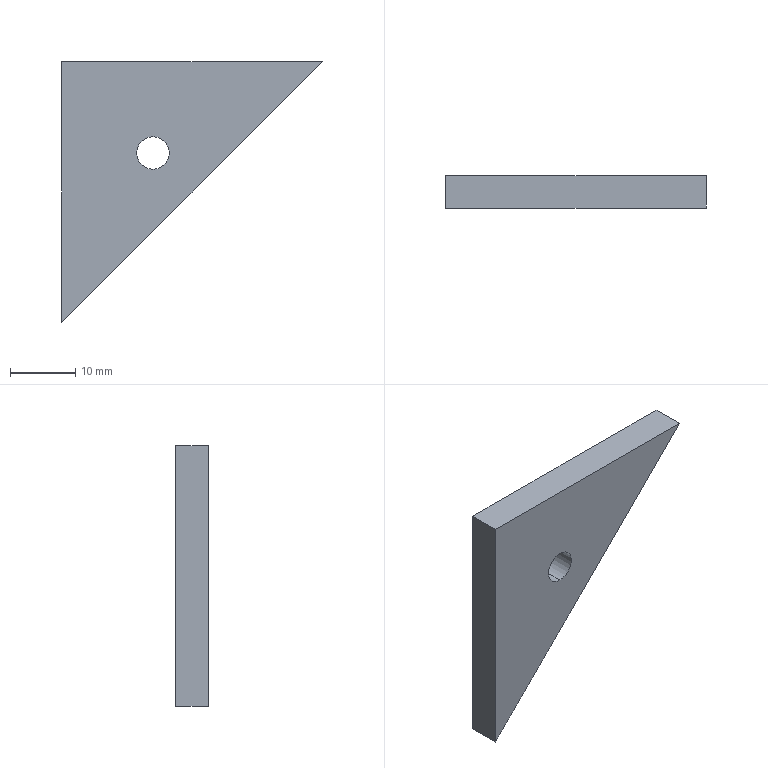Part | SolidWorks | features Extrusion 1, HoleWzd 1 | 1 solid | 7 faces | box 40 x 5 x 40 mm | volume 3902 mm3 | plane 5 | cylinder 2 | commonest cylinder face diameters 5 x2
STEP:
#1=CARTESIAN_POINT('',(14.,0.,-16.5));
#2=VERTEX_POINT('',#1);
#3=CARTESIAN_POINT('',(14.,0.,-11.5));
#4=VERTEX_POINT('',#3);
#5=CARTESIAN_POINT('',(14.,0.,-14.));
#6=DIRECTION('',(0.,1.,0.));
#7=DIRECTION('',(0.,0.,1.));
#8=AXIS2_PLACEMENT_3D('',#5,#6,#7);
#9=CIRCLE('',#8,2.5);
#10=EDGE_CURVE('',#2,#4,#9,.T.);
#11=ORIENTED_EDGE('',*,*,#10,.F.);
#12=CARTESIAN_POINT('',(14.,5.,-16.5));
#13=VERTEX_POINT('',#12);
#14=CARTESIAN_POINT('',(14.,5.,-16.5));
#15=DIRECTION('',(0.,1.,0.));
#16=VECTOR('',#15,1000.);
#17=LINE('',#14,#16);
#18=EDGE_CURVE('',#2,#13,#17,.T.);
#19=ORIENTED_EDGE('',*,*,#18,.T.);
#20=CARTESIAN_POINT('',(14.,5.,-11.5));
#21=VERTEX_POINT('',#20);
#22=CARTESIAN_POINT('',(14.,5.,-14.));
#23=DIRECTION('',(0.,1.,0.));
#24=DIRECTION('',(0.,0.,1.));
#25=AXIS2_PLACEMENT_3D('',#22,#23,#24);
#26=CIRCLE('',#25,2.5);
#27=EDGE_CURVE('',#13,#21,#26,.T.);
#28=ORIENTED_EDGE('',*,*,#27,.T.);
#29=CARTESIAN_POINT('',(14.,5.,-11.5));
#30=DIRECTION('',(0.,1.,0.));
#31=VECTOR('',#30,1000.);
#32=LINE('',#29,#31);
#33=EDGE_CURVE('',#4,#21,#32,.T.);
#34=ORIENTED_EDGE('',*,*,#33,.F.);
#35=EDGE_LOOP('',(#11,#19,#28,#34));
#36=FACE_OUTER_BOUND('',#35,.T.);
#37=CARTESIAN_POINT('',(14.,5.,-14.));
#38=DIRECTION('',(0.,1.,0.));
#39=DIRECTION('',(0.,0.,1.));
#40=AXIS2_PLACEMENT_3D('',#37,#38,#39);
#41=CYLINDRICAL_SURFACE('',#40,2.5);
#42=ADVANCED_FACE('',(#36),#41,.F.);
#43=CARTESIAN_POINT('',(40.,0.,0.));
#44=VERTEX_POINT('',#43);
#45=CARTESIAN_POINT('',(0.,0.,-40.));
#46=VERTEX_POINT('',#45);
#47=CARTESIAN_POINT('',(40.,0.,0.));
#48=DIRECTION('',(-0.7071,0.,-0.7071));
#49=VECTOR('',#48,1000.);
#50=LINE('',#47,#49);
#51=EDGE_CURVE('',#44,#46,#50,.T.);
#52=ORIENTED_EDGE('',*,*,#51,.T.);
#53=CARTESIAN_POINT('',(0.,5.,-40.));
#54=VERTEX_POINT('',#53);
#55=CARTESIAN_POINT('',(0.,5.,-40.));
#56=DIRECTION('',(0.,-1.,0.));
#57=VECTOR('',#56,1000.);
#58=LINE('',#55,#57);
#59=EDGE_CURVE('',#54,#46,#58,.T.);
#60=ORIENTED_EDGE('',*,*,#59,.F.);
#61=CARTESIAN_POINT('',(40.,5.,0.));
#62=VERTEX_POINT('',#61);
#63=CARTESIAN_POINT('',(40.,5.,0.));
#64=DIRECTION('',(-0.7071,0.,-0.7071));
#65=VECTOR('',#64,1000.);
#66=LINE('',#63,#65);
#67=EDGE_CURVE('',#62,#54,#66,.T.);
#68=ORIENTED_EDGE('',*,*,#67,.F.);
#69=CARTESIAN_POINT('',(40.,5.,0.));
#70=DIRECTION('',(0.,-1.,0.));
#71=VECTOR('',#70,1000.);
#72=LINE('',#69,#71);
#73=EDGE_CURVE('',#62,#44,#72,.T.);
#74=ORIENTED_EDGE('',*,*,#73,.T.);
#75=EDGE_LOOP('',(#52,#60,#68,#74));
#76=FACE_OUTER_BOUND('',#75,.T.);
#77=CARTESIAN_POINT('',(40.,5.,0.));
#78=DIRECTION('',(-0.7071,0.,0.7071));
#79=DIRECTION('',(0.7071,0.,0.7071));
#80=AXIS2_PLACEMENT_3D('',#77,#78,#79);
#81=PLANE('',#80);
#82=ADVANCED_FACE('',(#76),#81,.F.);
#83=CARTESIAN_POINT('',(0.,0.,0.));
#84=VERTEX_POINT('',#83);
#85=CARTESIAN_POINT('',(0.,0.,-40.));
#86=DIRECTION('',(0.,0.,1.));
#87=VECTOR('',#86,1000.);
#88=LINE('',#85,#87);
#89=EDGE_CURVE('',#46,#84,#88,.T.);
#90=ORIENTED_EDGE('',*,*,#89,.T.);
#91=CARTESIAN_POINT('',(0.,5.,0.));
#92=VERTEX_POINT('',#91);
#93=CARTESIAN_POINT('',(0.,5.,0.));
#94=DIRECTION('',(0.,-1.,0.));
#95=VECTOR('',#94,1000.);
#96=LINE('',#93,#95);
#97=EDGE_CURVE('',#92,#84,#96,.T.);
#98=ORIENTED_EDGE('',*,*,#97,.F.);
#99=CARTESIAN_POINT('',(0.,5.,-40.));
#100=DIRECTION('',(0.,0.,1.));
#101=VECTOR('',#100,1000.);
#102=LINE('',#99,#101);
#103=EDGE_CURVE('',#54,#92,#102,.T.);
#104=ORIENTED_EDGE('',*,*,#103,.F.);
#105=ORIENTED_EDGE('',*,*,#59,.T.);
#106=EDGE_LOOP('',(#90,#98,#104,#105));
#107=FACE_OUTER_BOUND('',#106,.T.);
#108=CARTESIAN_POINT('',(0.,5.,-40.));
#109=DIRECTION('',(1.,0.,0.));
#110=DIRECTION('',(0.,0.,-1.));
#111=AXIS2_PLACEMENT_3D('',#108,#109,#110);
#112=PLANE('',#111);
#113=ADVANCED_FACE('',(#107),#112,.F.);
#114=CARTESIAN_POINT('',(0.,0.,0.));
#115=DIRECTION('',(1.,0.,0.));
#116=VECTOR('',#115,1000.);
#117=LINE('',#114,#116);
#118=EDGE_CURVE('',#84,#44,#117,.T.);
#119=ORIENTED_EDGE('',*,*,#118,.T.);
#120=ORIENTED_EDGE('',*,*,#73,.F.);
#121=CARTESIAN_POINT('',(0.,5.,0.));
#122=DIRECTION('',(1.,0.,0.));
#123=VECTOR('',#122,1000.);
#124=LINE('',#121,#123);
#125=EDGE_CURVE('',#92,#62,#124,.T.);
#126=ORIENTED_EDGE('',*,*,#125,.F.);
#127=ORIENTED_EDGE('',*,*,#97,.T.);
#128=EDGE_LOOP('',(#119,#120,#126,#127));
#129=FACE_OUTER_BOUND('',#128,.T.);
#130=CARTESIAN_POINT('',(0.,5.,0.));
#131=DIRECTION('',(0.,0.,-1.));
#132=DIRECTION('',(-1.,0.,0.));
#133=AXIS2_PLACEMENT_3D('',#130,#131,#132);
#134=PLANE('',#133);
#135=ADVANCED_FACE('',(#129),#134,.F.);
#136=CARTESIAN_POINT('',(14.,5.,-14.));
#137=DIRECTION('',(0.,1.,0.));
#138=DIRECTION('',(0.,0.,1.));
#139=AXIS2_PLACEMENT_3D('',#136,#137,#138);
#140=CIRCLE('',#139,2.5);
#141=EDGE_CURVE('',#21,#13,#140,.T.);
#142=ORIENTED_EDGE('',*,*,#141,.F.);
#143=ORIENTED_EDGE('',*,*,#27,.F.);
#144=EDGE_LOOP('',(#142,#143));
#145=FACE_BOUND('',#144,.T.);
#146=ORIENTED_EDGE('',*,*,#67,.T.);
#147=ORIENTED_EDGE('',*,*,#103,.T.);
#148=ORIENTED_EDGE('',*,*,#125,.T.);
#149=EDGE_LOOP('',(#146,#147,#148));
#150=FACE_OUTER_BOUND('',#149,.T.);
#151=CARTESIAN_POINT('',(0.,5.,0.));
#152=DIRECTION('',(0.,1.,0.));
#153=DIRECTION('',(0.,0.,1.));
#154=AXIS2_PLACEMENT_3D('',#151,#152,#153);
#155=PLANE('',#154);
#156=ADVANCED_FACE('',(#145,#150),#155,.T.);
#157=CARTESIAN_POINT('',(14.,0.,-14.));
#158=DIRECTION('',(0.,1.,0.));
#159=DIRECTION('',(0.,0.,1.));
#160=AXIS2_PLACEMENT_3D('',#157,#158,#159);
#161=CIRCLE('',#160,2.5);
#162=EDGE_CURVE('',#4,#2,#161,.T.);
#163=ORIENTED_EDGE('',*,*,#162,.T.);
#164=ORIENTED_EDGE('',*,*,#10,.T.);
#165=EDGE_LOOP('',(#163,#164));
#166=FACE_BOUND('',#165,.T.);
#167=ORIENTED_EDGE('',*,*,#51,.F.);
#168=ORIENTED_EDGE('',*,*,#118,.F.);
#169=ORIENTED_EDGE('',*,*,#89,.F.);
#170=EDGE_LOOP('',(#167,#168,#169));
#171=FACE_OUTER_BOUND('',#170,.T.);
#172=CARTESIAN_POINT('',(0.,0.,0.));
#173=DIRECTION('',(0.,1.,0.));
#174=DIRECTION('',(0.,0.,1.));
#175=AXIS2_PLACEMENT_3D('',#172,#173,#174);
#176=PLANE('',#175);
#177=ADVANCED_FACE('',(#166,#171),#176,.F.);
#178=ORIENTED_EDGE('',*,*,#18,.F.);
#179=ORIENTED_EDGE('',*,*,#162,.F.);
#180=ORIENTED_EDGE('',*,*,#33,.T.);
#181=ORIENTED_EDGE('',*,*,#141,.T.);
#182=EDGE_LOOP('',(#178,#179,#180,#181));
#183=FACE_OUTER_BOUND('',#182,.T.);
#184=CARTESIAN_POINT('',(14.,5.,-14.));
#185=DIRECTION('',(0.,1.,0.));
#186=DIRECTION('',(0.,0.,1.));
#187=AXIS2_PLACEMENT_3D('',#184,#185,#186);
#188=CYLINDRICAL_SURFACE('',#187,2.5);
#189=ADVANCED_FACE('',(#183),#188,.F.);
#190=CLOSED_SHELL('',(#42,#82,#113,#135,#156,#177,#189));
#191=MANIFOLD_SOLID_BREP('',#190);
#192=CARTESIAN_POINT('',(0.,0.,0.));
#193=DIRECTION('',(0.,0.,1.));
#194=DIRECTION('',(1.,0.,0.));
#195=AXIS2_PLACEMENT_3D('',#192,#193,#194);
#196=(LENGTH_UNIT()NAMED_UNIT(*)SI_UNIT(.MILLI.,.METRE.));
#197=UNCERTAINTY_MEASURE_WITH_UNIT(LENGTH_MEASURE(0.00001),#196,'','');
#198=(NAMED_UNIT(*)PLANE_ANGLE_UNIT()SI_UNIT($,.RADIAN.));
#199=(NAMED_UNIT(*)SI_UNIT($,.STERADIAN.)SOLID_ANGLE_UNIT());
#200=(GEOMETRIC_REPRESENTATION_CONTEXT(3)GLOBAL_UNCERTAINTY_ASSIGNED_CONTEXT((#197))GLOBAL_UNIT_ASSIGNED_CONTEXT((#196,#198,#199))REPRESENTATION_CONTEXT('',''));
#201=ADVANCED_BREP_SHAPE_REPRESENTATION('',(#191,#195),#200);